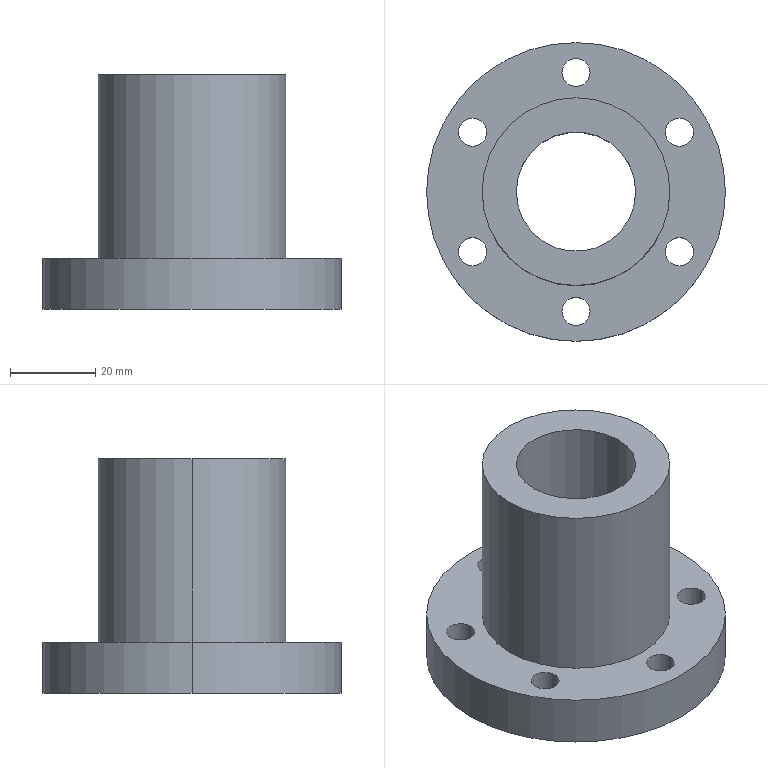Part | SolidWorks | features BaseBody 1 | 1 solid | 39 faces | box 70 x 70 x 55 mm | volume 72753 mm3 | cylinder 30 | plane 9 | commonest cylinder face diameters 6.6 x12 11 x12 28 x2 44 x2 70 x2
STEP:
#1=CARTESIAN_POINT('',(-24.249,19.5,6.8));
#2=VERTEX_POINT('',#1);
#3=CARTESIAN_POINT('',(-24.249,8.5,6.8));
#4=VERTEX_POINT('',#3);
#5=CARTESIAN_POINT('',(-24.249,14.,6.8));
#6=DIRECTION('',(0.,0.,1.));
#7=DIRECTION('',(0.,1.,0.));
#8=AXIS2_PLACEMENT_3D('',#5,#6,#7);
#9=CIRCLE('',#8,5.5);
#10=EDGE_CURVE('',#2,#4,#9,.T.);
#11=ORIENTED_EDGE('',*,*,#10,.T.);
#12=CARTESIAN_POINT('',(-24.249,8.5,0.));
#13=VERTEX_POINT('',#12);
#14=CARTESIAN_POINT('',(-24.249,8.5,6.8));
#15=DIRECTION('',(0.,0.,-1.));
#16=VECTOR('',#15,1000.);
#17=LINE('',#14,#16);
#18=EDGE_CURVE('',#4,#13,#17,.T.);
#19=ORIENTED_EDGE('',*,*,#18,.T.);
#20=CARTESIAN_POINT('',(-24.249,19.5,0.));
#21=VERTEX_POINT('',#20);
#22=CARTESIAN_POINT('',(-24.249,14.,0.));
#23=DIRECTION('',(0.,0.,-1.));
#24=DIRECTION('',(0.,1.,0.));
#25=AXIS2_PLACEMENT_3D('',#22,#23,#24);
#26=CIRCLE('',#25,5.5);
#27=EDGE_CURVE('',#13,#21,#26,.T.);
#28=ORIENTED_EDGE('',*,*,#27,.T.);
#29=CARTESIAN_POINT('',(-24.249,19.5,6.8));
#30=DIRECTION('',(0.,0.,-1.));
#31=VECTOR('',#30,1000.);
#32=LINE('',#29,#31);
#33=EDGE_CURVE('',#2,#21,#32,.T.);
#34=ORIENTED_EDGE('',*,*,#33,.F.);
#35=EDGE_LOOP('',(#11,#19,#28,#34));
#36=FACE_OUTER_BOUND('',#35,.T.);
#37=CARTESIAN_POINT('',(-24.249,14.,6.8));
#38=DIRECTION('',(0.,0.,-1.));
#39=DIRECTION('',(0.,1.,0.));
#40=AXIS2_PLACEMENT_3D('',#37,#38,#39);
#41=CYLINDRICAL_SURFACE('',#40,5.5);
#42=ADVANCED_FACE('',(#36),#41,.F.);
#43=CARTESIAN_POINT('',(-14.,0.,55.));
#44=VERTEX_POINT('',#43);
#45=CARTESIAN_POINT('',(14.,0.,55.));
#46=VERTEX_POINT('',#45);
#47=CARTESIAN_POINT('',(0.,0.,55.));
#48=DIRECTION('',(0.,0.,1.));
#49=DIRECTION('',(-1.,0.,0.));
#50=AXIS2_PLACEMENT_3D('',#47,#48,#49);
#51=CIRCLE('',#50,14.);
#52=EDGE_CURVE('',#44,#46,#51,.T.);
#53=ORIENTED_EDGE('',*,*,#52,.T.);
#54=CARTESIAN_POINT('',(14.,0.,0.));
#55=VERTEX_POINT('',#54);
#56=CARTESIAN_POINT('',(14.,0.,55.));
#57=DIRECTION('',(0.,0.,-1.));
#58=VECTOR('',#57,1000.);
#59=LINE('',#56,#58);
#60=EDGE_CURVE('',#46,#55,#59,.T.);
#61=ORIENTED_EDGE('',*,*,#60,.T.);
#62=CARTESIAN_POINT('',(-14.,0.,0.));
#63=VERTEX_POINT('',#62);
#64=CARTESIAN_POINT('',(0.,0.,0.));
#65=DIRECTION('',(0.,0.,-1.));
#66=DIRECTION('',(-1.,0.,0.));
#67=AXIS2_PLACEMENT_3D('',#64,#65,#66);
#68=CIRCLE('',#67,14.);
#69=EDGE_CURVE('',#55,#63,#68,.T.);
#70=ORIENTED_EDGE('',*,*,#69,.T.);
#71=CARTESIAN_POINT('',(-14.,0.,55.));
#72=DIRECTION('',(0.,0.,-1.));
#73=VECTOR('',#72,1000.);
#74=LINE('',#71,#73);
#75=EDGE_CURVE('',#44,#63,#74,.T.);
#76=ORIENTED_EDGE('',*,*,#75,.F.);
#77=EDGE_LOOP('',(#53,#61,#70,#76));
#78=FACE_OUTER_BOUND('',#77,.T.);
#79=CARTESIAN_POINT('',(0.,0.,55.));
#80=DIRECTION('',(0.,0.,-1.));
#81=DIRECTION('',(-1.,0.,0.));
#82=AXIS2_PLACEMENT_3D('',#79,#80,#81);
#83=CYLINDRICAL_SURFACE('',#82,14.);
#84=ADVANCED_FACE('',(#78),#83,.F.);
#85=CARTESIAN_POINT('',(0.,33.5,6.8));
#86=VERTEX_POINT('',#85);
#87=CARTESIAN_POINT('',(0.,22.5,6.8));
#88=VERTEX_POINT('',#87);
#89=CARTESIAN_POINT('',(0.,28.,6.8));
#90=DIRECTION('',(0.,0.,1.));
#91=DIRECTION('',(0.,1.,0.));
#92=AXIS2_PLACEMENT_3D('',#89,#90,#91);
#93=CIRCLE('',#92,5.5);
#94=EDGE_CURVE('',#86,#88,#93,.T.);
#95=ORIENTED_EDGE('',*,*,#94,.T.);
#96=CARTESIAN_POINT('',(0.,22.5,0.));
#97=VERTEX_POINT('',#96);
#98=CARTESIAN_POINT('',(0.,22.5,6.8));
#99=DIRECTION('',(0.,0.,-1.));
#100=VECTOR('',#99,1000.);
#101=LINE('',#98,#100);
#102=EDGE_CURVE('',#88,#97,#101,.T.);
#103=ORIENTED_EDGE('',*,*,#102,.T.);
#104=CARTESIAN_POINT('',(0.,33.5,0.));
#105=VERTEX_POINT('',#104);
#106=CARTESIAN_POINT('',(0.,28.,0.));
#107=DIRECTION('',(0.,0.,-1.));
#108=DIRECTION('',(0.,1.,0.));
#109=AXIS2_PLACEMENT_3D('',#106,#107,#108);
#110=CIRCLE('',#109,5.5);
#111=EDGE_CURVE('',#97,#105,#110,.T.);
#112=ORIENTED_EDGE('',*,*,#111,.T.);
#113=CARTESIAN_POINT('',(0.,33.5,6.8));
#114=DIRECTION('',(0.,0.,-1.));
#115=VECTOR('',#114,1000.);
#116=LINE('',#113,#115);
#117=EDGE_CURVE('',#86,#105,#116,.T.);
#118=ORIENTED_EDGE('',*,*,#117,.F.);
#119=EDGE_LOOP('',(#95,#103,#112,#118));
#120=FACE_OUTER_BOUND('',#119,.T.);
#121=CARTESIAN_POINT('',(0.,28.,6.8));
#122=DIRECTION('',(0.,0.,-1.));
#123=DIRECTION('',(0.,1.,0.));
#124=AXIS2_PLACEMENT_3D('',#121,#122,#123);
#125=CYLINDRICAL_SURFACE('',#124,5.5);
#126=ADVANCED_FACE('',(#120),#125,.F.);
#127=CARTESIAN_POINT('',(24.249,19.5,6.8));
#128=VERTEX_POINT('',#127);
#129=CARTESIAN_POINT('',(24.249,8.5,6.8));
#130=VERTEX_POINT('',#129);
#131=CARTESIAN_POINT('',(24.249,14.,6.8));
#132=DIRECTION('',(0.,0.,1.));
#133=DIRECTION('',(0.,1.,0.));
#134=AXIS2_PLACEMENT_3D('',#131,#132,#133);
#135=CIRCLE('',#134,5.5);
#136=EDGE_CURVE('',#128,#130,#135,.T.);
#137=ORIENTED_EDGE('',*,*,#136,.T.);
#138=CARTESIAN_POINT('',(24.249,8.5,0.));
#139=VERTEX_POINT('',#138);
#140=CARTESIAN_POINT('',(24.249,8.5,6.8));
#141=DIRECTION('',(0.,0.,-1.));
#142=VECTOR('',#141,1000.);
#143=LINE('',#140,#142);
#144=EDGE_CURVE('',#130,#139,#143,.T.);
#145=ORIENTED_EDGE('',*,*,#144,.T.);
#146=CARTESIAN_POINT('',(24.249,19.5,0.));
#147=VERTEX_POINT('',#146);
#148=CARTESIAN_POINT('',(24.249,14.,0.));
#149=DIRECTION('',(0.,0.,-1.));
#150=DIRECTION('',(0.,1.,0.));
#151=AXIS2_PLACEMENT_3D('',#148,#149,#150);
#152=CIRCLE('',#151,5.5);
#153=EDGE_CURVE('',#139,#147,#152,.T.);
#154=ORIENTED_EDGE('',*,*,#153,.T.);
#155=CARTESIAN_POINT('',(24.249,19.5,6.8));
#156=DIRECTION('',(0.,0.,-1.));
#157=VECTOR('',#156,1000.);
#158=LINE('',#155,#157);
#159=EDGE_CURVE('',#128,#147,#158,.T.);
#160=ORIENTED_EDGE('',*,*,#159,.F.);
#161=EDGE_LOOP('',(#137,#145,#154,#160));
#162=FACE_OUTER_BOUND('',#161,.T.);
#163=CARTESIAN_POINT('',(24.249,14.,6.8));
#164=DIRECTION('',(0.,0.,-1.));
#165=DIRECTION('',(0.,1.,0.));
#166=AXIS2_PLACEMENT_3D('',#163,#164,#165);
#167=CYLINDRICAL_SURFACE('',#166,5.5);
#168=ADVANCED_FACE('',(#162),#167,.F.);
#169=CARTESIAN_POINT('',(24.249,-8.5,6.8));
#170=VERTEX_POINT('',#169);
#171=CARTESIAN_POINT('',(24.249,-19.5,6.8));
#172=VERTEX_POINT('',#171);
#173=CARTESIAN_POINT('',(24.249,-14.,6.8));
#174=DIRECTION('',(0.,0.,1.));
#175=DIRECTION('',(0.,1.,0.));
#176=AXIS2_PLACEMENT_3D('',#173,#174,#175);
#177=CIRCLE('',#176,5.5);
#178=EDGE_CURVE('',#170,#172,#177,.T.);
#179=ORIENTED_EDGE('',*,*,#178,.T.);
#180=CARTESIAN_POINT('',(24.249,-19.5,0.));
#181=VERTEX_POINT('',#180);
#182=CARTESIAN_POINT('',(24.249,-19.5,6.8));
#183=DIRECTION('',(0.,0.,-1.));
#184=VECTOR('',#183,1000.);
#185=LINE('',#182,#184);
#186=EDGE_CURVE('',#172,#181,#185,.T.);
#187=ORIENTED_EDGE('',*,*,#186,.T.);
#188=CARTESIAN_POINT('',(24.249,-8.5,0.));
#189=VERTEX_POINT('',#188);
#190=CARTESIAN_POINT('',(24.249,-14.,0.));
#191=DIRECTION('',(0.,0.,-1.));
#192=DIRECTION('',(0.,1.,0.));
#193=AXIS2_PLACEMENT_3D('',#190,#191,#192);
#194=CIRCLE('',#193,5.5);
#195=EDGE_CURVE('',#181,#189,#194,.T.);
#196=ORIENTED_EDGE('',*,*,#195,.T.);
#197=CARTESIAN_POINT('',(24.249,-8.5,6.8));
#198=DIRECTION('',(0.,0.,-1.));
#199=VECTOR('',#198,1000.);
#200=LINE('',#197,#199);
#201=EDGE_CURVE('',#170,#189,#200,.T.);
#202=ORIENTED_EDGE('',*,*,#201,.F.);
#203=EDGE_LOOP('',(#179,#187,#196,#202));
#204=FACE_OUTER_BOUND('',#203,.T.);
#205=CARTESIAN_POINT('',(24.249,-14.,6.8));
#206=DIRECTION('',(0.,0.,-1.));
#207=DIRECTION('',(0.,1.,0.));
#208=AXIS2_PLACEMENT_3D('',#205,#206,#207);
#209=CYLINDRICAL_SURFACE('',#208,5.5);
#210=ADVANCED_FACE('',(#204),#209,.F.);
#211=CARTESIAN_POINT('',(0.,-22.5,6.8));
#212=VERTEX_POINT('',#211);
#213=CARTESIAN_POINT('',(0.,-33.5,6.8));
#214=VERTEX_POINT('',#213);
#215=CARTESIAN_POINT('',(0.,-28.,6.8));
#216=DIRECTION('',(0.,0.,1.));
#217=DIRECTION('',(0.,1.,0.));
#218=AXIS2_PLACEMENT_3D('',#215,#216,#217);
#219=CIRCLE('',#218,5.5);
#220=EDGE_CURVE('',#212,#214,#219,.T.);
#221=ORIENTED_EDGE('',*,*,#220,.T.);
#222=CARTESIAN_POINT('',(0.,-33.5,0.));
#223=VERTEX_POINT('',#222);
#224=CARTESIAN_POINT('',(0.,-33.5,6.8));
#225=DIRECTION('',(0.,0.,-1.));
#226=VECTOR('',#225,1000.);
#227=LINE('',#224,#226);
#228=EDGE_CURVE('',#214,#223,#227,.T.);
#229=ORIENTED_EDGE('',*,*,#228,.T.);
#230=CARTESIAN_POINT('',(0.,-22.5,0.));
#231=VERTEX_POINT('',#230);
#232=CARTESIAN_POINT('',(0.,-28.,0.));
#233=DIRECTION('',(0.,0.,-1.));
#234=DIRECTION('',(0.,1.,0.));
#235=AXIS2_PLACEMENT_3D('',#232,#233,#234);
#236=CIRCLE('',#235,5.5);
#237=EDGE_CURVE('',#223,#231,#236,.T.);
#238=ORIENTED_EDGE('',*,*,#237,.T.);
#239=CARTESIAN_POINT('',(0.,-22.5,6.8));
#240=DIRECTION('',(0.,0.,-1.));
#241=VECTOR('',#240,1000.);
#242=LINE('',#239,#241);
#243=EDGE_CURVE('',#212,#231,#242,.T.);
#244=ORIENTED_EDGE('',*,*,#243,.F.);
#245=EDGE_LOOP('',(#221,#229,#238,#244));
#246=FACE_OUTER_BOUND('',#245,.T.);
#247=CARTESIAN_POINT('',(0.,-28.,6.8));
#248=DIRECTION('',(0.,0.,-1.));
#249=DIRECTION('',(0.,1.,0.));
#250=AXIS2_PLACEMENT_3D('',#247,#248,#249);
#251=CYLINDRICAL_SURFACE('',#250,5.5);
#252=ADVANCED_FACE('',(#246),#251,.F.);
#253=CARTESIAN_POINT('',(-24.249,-8.5,6.8));
#254=VERTEX_POINT('',#253);
#255=CARTESIAN_POINT('',(-24.249,-19.5,6.8));
#256=VERTEX_POINT('',#255);
#257=CARTESIAN_POINT('',(-24.249,-14.,6.8));
#258=DIRECTION('',(0.,0.,1.));
#259=DIRECTION('',(0.,1.,0.));
#260=AXIS2_PLACEMENT_3D('',#257,#258,#259);
#261=CIRCLE('',#260,5.5);
#262=EDGE_CURVE('',#254,#256,#261,.T.);
#263=ORIENTED_EDGE('',*,*,#262,.T.);
#264=CARTESIAN_POINT('',(-24.249,-19.5,0.));
#265=VERTEX_POINT('',#264);
#266=CARTESIAN_POINT('',(-24.249,-19.5,6.8));
#267=DIRECTION('',(0.,0.,-1.));
#268=VECTOR('',#267,1000.);
#269=LINE('',#266,#268);
#270=EDGE_CURVE('',#256,#265,#269,.T.);
#271=ORIENTED_EDGE('',*,*,#270,.T.);
#272=CARTESIAN_POINT('',(-24.249,-8.5,0.));
#273=VERTEX_POINT('',#272);
#274=CARTESIAN_POINT('',(-24.249,-14.,0.));
#275=DIRECTION('',(0.,0.,-1.));
#276=DIRECTION('',(0.,1.,0.));
#277=AXIS2_PLACEMENT_3D('',#274,#275,#276);
#278=CIRCLE('',#277,5.5);
#279=EDGE_CURVE('',#265,#273,#278,.T.);
#280=ORIENTED_EDGE('',*,*,#279,.T.);
#281=CARTESIAN_POINT('',(-24.249,-8.5,6.8));
#282=DIRECTION('',(0.,0.,-1.));
#283=VECTOR('',#282,1000.);
#284=LINE('',#281,#283);
#285=EDGE_CURVE('',#254,#273,#284,.T.);
#286=ORIENTED_EDGE('',*,*,#285,.F.);
#287=EDGE_LOOP('',(#263,#271,#280,#286));
#288=FACE_OUTER_BOUND('',#287,.T.);
#289=CARTESIAN_POINT('',(-24.249,-14.,6.8));
#290=DIRECTION('',(0.,0.,-1.));
#291=DIRECTION('',(0.,1.,0.));
#292=AXIS2_PLACEMENT_3D('',#289,#290,#291);
#293=CYLINDRICAL_SURFACE('',#292,5.5);
#294=ADVANCED_FACE('',(#288),#293,.F.);
#295=CARTESIAN_POINT('',(35.,0.,12.));
#296=VERTEX_POINT('',#295);
#297=CARTESIAN_POINT('',(-35.,0.,12.));
#298=VERTEX_POINT('',#297);
#299=CARTESIAN_POINT('',(0.,0.,12.));
#300=DIRECTION('',(0.,0.,1.));
#301=DIRECTION('',(-1.,0.,0.));
#302=AXIS2_PLACEMENT_3D('',#299,#300,#301);
#303=CIRCLE('',#302,35.);
#304=EDGE_CURVE('',#296,#298,#303,.T.);
#305=ORIENTED_EDGE('',*,*,#304,.F.);
#306=CARTESIAN_POINT('',(35.,0.,0.));
#307=VERTEX_POINT('',#306);
#308=CARTESIAN_POINT('',(35.,0.,12.));
#309=DIRECTION('',(0.,0.,-1.));
#310=VECTOR('',#309,1000.);
#311=LINE('',#308,#310);
#312=EDGE_CURVE('',#296,#307,#311,.T.);
#313=ORIENTED_EDGE('',*,*,#312,.T.);
#314=CARTESIAN_POINT('',(-35.,0.,0.));
#315=VERTEX_POINT('',#314);
#316=CARTESIAN_POINT('',(0.,0.,0.));
#317=DIRECTION('',(0.,0.,1.));
#318=DIRECTION('',(-1.,0.,0.));
#319=AXIS2_PLACEMENT_3D('',#316,#317,#318);
#320=CIRCLE('',#319,35.);
#321=EDGE_CURVE('',#307,#315,#320,.T.);
#322=ORIENTED_EDGE('',*,*,#321,.T.);
#323=CARTESIAN_POINT('',(-35.,0.,12.));
#324=DIRECTION('',(0.,0.,-1.));
#325=VECTOR('',#324,1000.);
#326=LINE('',#323,#325);
#327=EDGE_CURVE('',#298,#315,#326,.T.);
#328=ORIENTED_EDGE('',*,*,#327,.F.);
#329=EDGE_LOOP('',(#305,#313,#322,#328));
#330=FACE_OUTER_BOUND('',#329,.T.);
#331=CARTESIAN_POINT('',(0.,0.,12.));
#332=DIRECTION('',(0.,0.,-1.));
#333=DIRECTION('',(-1.,0.,0.));
#334=AXIS2_PLACEMENT_3D('',#331,#332,#333);
#335=CYLINDRICAL_SURFACE('',#334,35.);
#336=ADVANCED_FACE('',(#330),#335,.T.);
#337=CARTESIAN_POINT('',(-27.549,14.,12.));
#338=VERTEX_POINT('',#337);
#339=CARTESIAN_POINT('',(-20.949,14.,12.));
#340=VERTEX_POINT('',#339);
#341=CARTESIAN_POINT('',(-24.249,14.,12.));
#342=DIRECTION('',(0.,0.,1.));
#343=DIRECTION('',(-1.,0.,0.));
#344=AXIS2_PLACEMENT_3D('',#341,#342,#343);
#345=CIRCLE('',#344,3.3);
#346=EDGE_CURVE('',#338,#340,#345,.T.);
#347=ORIENTED_EDGE('',*,*,#346,.T.);
#348=CARTESIAN_POINT('',(-20.949,14.,6.8));
#349=VERTEX_POINT('',#348);
#350=CARTESIAN_POINT('',(-20.949,14.,12.));
#351=DIRECTION('',(0.,0.,-1.));
#352=VECTOR('',#351,1000.);
#353=LINE('',#350,#352);
#354=EDGE_CURVE('',#340,#349,#353,.T.);
#355=ORIENTED_EDGE('',*,*,#354,.T.);
#356=CARTESIAN_POINT('',(-27.549,14.,6.8));
#357=VERTEX_POINT('',#356);
#358=CARTESIAN_POINT('',(-24.249,14.,6.8));
#359=DIRECTION('',(0.,0.,-1.));
#360=DIRECTION('',(-1.,0.,0.));
#361=AXIS2_PLACEMENT_3D('',#358,#359,#360);
#362=CIRCLE('',#361,3.3);
#363=EDGE_CURVE('',#349,#357,#362,.T.);
#364=ORIENTED_EDGE('',*,*,#363,.T.);
#365=CARTESIAN_POINT('',(-27.549,14.,12.));
#366=DIRECTION('',(0.,0.,-1.));
#367=VECTOR('',#366,1000.);
#368=LINE('',#365,#367);
#369=EDGE_CURVE('',#338,#357,#368,.T.);
#370=ORIENTED_EDGE('',*,*,#369,.F.);
#371=EDGE_LOOP('',(#347,#355,#364,#370));
#372=FACE_OUTER_BOUND('',#371,.T.);
#373=CARTESIAN_POINT('',(-24.249,14.,12.));
#374=DIRECTION('',(0.,0.,-1.));
#375=DIRECTION('',(-1.,0.,0.));
#376=AXIS2_PLACEMENT_3D('',#373,#374,#375);
#377=CYLINDRICAL_SURFACE('',#376,3.3);
#378=ADVANCED_FACE('',(#372),#377,.F.);
#379=CARTESIAN_POINT('',(22.,0.,55.));
#380=VERTEX_POINT('',#379);
#381=CARTESIAN_POINT('',(-22.,0.,55.));
#382=VERTEX_POINT('',#381);
#383=CARTESIAN_POINT('',(0.,0.,55.));
#384=DIRECTION('',(0.,0.,1.));
#385=DIRECTION('',(-1.,0.,0.));
#386=AXIS2_PLACEMENT_3D('',#383,#384,#385);
#387=CIRCLE('',#386,22.);
#388=EDGE_CURVE('',#380,#382,#387,.T.);
#389=ORIENTED_EDGE('',*,*,#388,.F.);
#390=CARTESIAN_POINT('',(22.,0.,12.));
#391=VERTEX_POINT('',#390);
#392=CARTESIAN_POINT('',(22.,0.,55.));
#393=DIRECTION('',(0.,0.,-1.));
#394=VECTOR('',#393,1000.);
#395=LINE('',#392,#394);
#396=EDGE_CURVE('',#380,#391,#395,.T.);
#397=ORIENTED_EDGE('',*,*,#396,.T.);
#398=CARTESIAN_POINT('',(-22.,0.,12.));
#399=VERTEX_POINT('',#398);
#400=CARTESIAN_POINT('',(0.,0.,12.));
#401=DIRECTION('',(0.,0.,-1.));
#402=DIRECTION('',(-1.,0.,0.));
#403=AXIS2_PLACEMENT_3D('',#400,#401,#402);
#404=CIRCLE('',#403,22.);
#405=EDGE_CURVE('',#399,#391,#404,.T.);
#406=ORIENTED_EDGE('',*,*,#405,.F.);
#407=CARTESIAN_POINT('',(-22.,0.,55.));
#408=DIRECTION('',(0.,0.,-1.));
#409=VECTOR('',#408,1000.);
#410=LINE('',#407,#409);
#411=EDGE_CURVE('',#382,#399,#410,.T.);
#412=ORIENTED_EDGE('',*,*,#411,.F.);
#413=EDGE_LOOP('',(#389,#397,#406,#412));
#414=FACE_OUTER_BOUND('',#413,.T.);
#415=CARTESIAN_POINT('',(0.,0.,55.));
#416=DIRECTION('',(0.,0.,-1.));
#417=DIRECTION('',(-1.,0.,0.));
#418=AXIS2_PLACEMENT_3D('',#415,#416,#417);
#419=CYLINDRICAL_SURFACE('',#418,22.);
#420=ADVANCED_FACE('',(#414),#419,.T.);
#421=CARTESIAN_POINT('',(3.3,28.,12.));
#422=VERTEX_POINT('',#421);
#423=CARTESIAN_POINT('',(-3.3,28.,12.));
#424=VERTEX_POINT('',#423);
#425=CARTESIAN_POINT('',(0.,28.,12.));
#426=DIRECTION('',(0.,0.,-1.));
#427=DIRECTION('',(-1.,0.,0.));
#428=AXIS2_PLACEMENT_3D('',#425,#426,#427);
#429=CIRCLE('',#428,3.3);
#430=EDGE_CURVE('',#422,#424,#429,.T.);
#431=ORIENTED_EDGE('',*,*,#430,.F.);
#432=CARTESIAN_POINT('',(3.3,28.,6.8));
#433=VERTEX_POINT('',#432);
#434=CARTESIAN_POINT('',(3.3,28.,12.));
#435=DIRECTION('',(0.,0.,-1.));
#436=VECTOR('',#435,1000.);
#437=LINE('',#434,#436);
#438=EDGE_CURVE('',#422,#433,#437,.T.);
#439=ORIENTED_EDGE('',*,*,#438,.T.);
#440=CARTESIAN_POINT('',(-3.3,28.,6.8));
#441=VERTEX_POINT('',#440);
#442=CARTESIAN_POINT('',(0.,28.,6.8));
#443=DIRECTION('',(0.,0.,-1.));
#444=DIRECTION('',(-1.,0.,0.));
#445=AXIS2_PLACEMENT_3D('',#442,#443,#444);
#446=CIRCLE('',#445,3.3);
#447=EDGE_CURVE('',#433,#441,#446,.T.);
#448=ORIENTED_EDGE('',*,*,#447,.T.);
#449=CARTESIAN_POINT('',(-3.3,28.,12.));
#450=DIRECTION('',(0.,0.,-1.));
#451=VECTOR('',#450,1000.);
#452=LINE('',#449,#451);
#453=EDGE_CURVE('',#424,#441,#452,.T.);
#454=ORIENTED_EDGE('',*,*,#453,.F.);
#455=EDGE_LOOP('',(#431,#439,#448,#454));
#456=FACE_OUTER_BOUND('',#455,.T.);
#457=CARTESIAN_POINT('',(0.,28.,12.));
#458=DIRECTION('',(0.,0.,-1.));
#459=DIRECTION('',(-1.,0.,0.));
#460=AXIS2_PLACEMENT_3D('',#457,#458,#459);
#461=CYLINDRICAL_SURFACE('',#460,3.3);
#462=ADVANCED_FACE('',(#456),#461,.F.);
#463=CARTESIAN_POINT('',(27.549,14.,12.));
#464=VERTEX_POINT('',#463);
#465=CARTESIAN_POINT('',(20.949,14.,12.));
#466=VERTEX_POINT('',#465);
#467=CARTESIAN_POINT('',(24.249,14.,12.));
#468=DIRECTION('',(0.,0.,-1.));
#469=DIRECTION('',(-1.,0.,0.));
#470=AXIS2_PLACEMENT_3D('',#467,#468,#469);
#471=CIRCLE('',#470,3.3);
#472=EDGE_CURVE('',#464,#466,#471,.T.);
#473=ORIENTED_EDGE('',*,*,#472,.F.);
#474=CARTESIAN_POINT('',(27.549,14.,6.8));
#475=VERTEX_POINT('',#474);
#476=CARTESIAN_POINT('',(27.549,14.,12.));
#477=DIRECTION('',(0.,0.,-1.));
#478=VECTOR('',#477,1000.);
#479=LINE('',#476,#478);
#480=EDGE_CURVE('',#464,#475,#479,.T.);
#481=ORIENTED_EDGE('',*,*,#480,.T.);
#482=CARTESIAN_POINT('',(20.949,14.,6.8));
#483=VERTEX_POINT('',#482);
#484=CARTESIAN_POINT('',(24.249,14.,6.8));
#485=DIRECTION('',(0.,0.,-1.));
#486=DIRECTION('',(-1.,0.,0.));
#487=AXIS2_PLACEMENT_3D('',#484,#485,#486);
#488=CIRCLE('',#487,3.3);
#489=EDGE_CURVE('',#475,#483,#488,.T.);
#490=ORIENTED_EDGE('',*,*,#489,.T.);
#491=CARTESIAN_POINT('',(20.949,14.,12.));
#492=DIRECTION('',(0.,0.,-1.));
#493=VECTOR('',#492,1000.);
#494=LINE('',#491,#493);
#495=EDGE_CURVE('',#466,#483,#494,.T.);
#496=ORIENTED_EDGE('',*,*,#495,.F.);
#497=EDGE_LOOP('',(#473,#481,#490,#496));
#498=FACE_OUTER_BOUND('',#497,.T.);
#499=CARTESIAN_POINT('',(24.249,14.,12.));
#500=DIRECTION('',(0.,0.,-1.));
#501=DIRECTION('',(-1.,0.,0.));
#502=AXIS2_PLACEMENT_3D('',#499,#500,#501);
#503=CYLINDRICAL_SURFACE('',#502,3.3);
#504=ADVANCED_FACE('',(#498),#503,.F.);
#505=CARTESIAN_POINT('',(27.549,-14.,12.));
#506=VERTEX_POINT('',#505);
#507=CARTESIAN_POINT('',(20.949,-14.,12.));
#508=VERTEX_POINT('',#507);
#509=CARTESIAN_POINT('',(24.249,-14.,12.));
#510=DIRECTION('',(0.,0.,-1.));
#511=DIRECTION('',(-1.,0.,0.));
#512=AXIS2_PLACEMENT_3D('',#509,#510,#511);
#513=CIRCLE('',#512,3.3);
#514=EDGE_CURVE('',#506,#508,#513,.T.);
#515=ORIENTED_EDGE('',*,*,#514,.F.);
#516=CARTESIAN_POINT('',(27.549,-14.,6.8));
#517=VERTEX_POINT('',#516);
#518=CARTESIAN_POINT('',(27.549,-14.,12.));
#519=DIRECTION('',(0.,0.,-1.));
#520=VECTOR('',#519,1000.);
#521=LINE('',#518,#520);
#522=EDGE_CURVE('',#506,#517,#521,.T.);
#523=ORIENTED_EDGE('',*,*,#522,.T.);
#524=CARTESIAN_POINT('',(20.949,-14.,6.8));
#525=VERTEX_POINT('',#524);
#526=CARTESIAN_POINT('',(24.249,-14.,6.8));
#527=DIRECTION('',(0.,0.,-1.));
#528=DIRECTION('',(-1.,0.,0.));
#529=AXIS2_PLACEMENT_3D('',#526,#527,#528);
#530=CIRCLE('',#529,3.3);
#531=EDGE_CURVE('',#517,#525,#530,.T.);
#532=ORIENTED_EDGE('',*,*,#531,.T.);
#533=CARTESIAN_POINT('',(20.949,-14.,12.));
#534=DIRECTION('',(0.,0.,-1.));
#535=VECTOR('',#534,1000.);
#536=LINE('',#533,#535);
#537=EDGE_CURVE('',#508,#525,#536,.T.);
#538=ORIENTED_EDGE('',*,*,#537,.F.);
#539=EDGE_LOOP('',(#515,#523,#532,#538));
#540=FACE_OUTER_BOUND('',#539,.T.);
#541=CARTESIAN_POINT('',(24.249,-14.,12.));
#542=DIRECTION('',(0.,0.,-1.));
#543=DIRECTION('',(-1.,0.,0.));
#544=AXIS2_PLACEMENT_3D('',#541,#542,#543);
#545=CYLINDRICAL_SURFACE('',#544,3.3);
#546=ADVANCED_FACE('',(#540),#545,.F.);
#547=CARTESIAN_POINT('',(3.3,-28.,12.));
#548=VERTEX_POINT('',#547);
#549=CARTESIAN_POINT('',(-3.3,-28.,12.));
#550=VERTEX_POINT('',#549);
#551=CARTESIAN_POINT('',(0.,-28.,12.));
#552=DIRECTION('',(0.,0.,-1.));
#553=DIRECTION('',(-1.,0.,0.));
#554=AXIS2_PLACEMENT_3D('',#551,#552,#553);
#555=CIRCLE('',#554,3.3);
#556=EDGE_CURVE('',#548,#550,#555,.T.);
#557=ORIENTED_EDGE('',*,*,#556,.F.);
#558=CARTESIAN_POINT('',(3.3,-28.,6.8));
#559=VERTEX_POINT('',#558);
#560=CARTESIAN_POINT('',(3.3,-28.,12.));
#561=DIRECTION('',(0.,0.,-1.));
#562=VECTOR('',#561,1000.);
#563=LINE('',#560,#562);
#564=EDGE_CURVE('',#548,#559,#563,.T.);
#565=ORIENTED_EDGE('',*,*,#564,.T.);
#566=CARTESIAN_POINT('',(-3.3,-28.,6.8));
#567=VERTEX_POINT('',#566);
#568=CARTESIAN_POINT('',(0.,-28.,6.8));
#569=DIRECTION('',(0.,0.,-1.));
#570=DIRECTION('',(-1.,0.,0.));
#571=AXIS2_PLACEMENT_3D('',#568,#569,#570);
#572=CIRCLE('',#571,3.3);
#573=EDGE_CURVE('',#559,#567,#572,.T.);
#574=ORIENTED_EDGE('',*,*,#573,.T.);
#575=CARTESIAN_POINT('',(-3.3,-28.,12.));
#576=DIRECTION('',(0.,0.,-1.));
#577=VECTOR('',#576,1000.);
#578=LINE('',#575,#577);
#579=EDGE_CURVE('',#550,#567,#578,.T.);
#580=ORIENTED_EDGE('',*,*,#579,.F.);
#581=EDGE_LOOP('',(#557,#565,#574,#580));
#582=FACE_OUTER_BOUND('',#581,.T.);
#583=CARTESIAN_POINT('',(0.,-28.,12.));
#584=DIRECTION('',(0.,0.,-1.));
#585=DIRECTION('',(-1.,0.,0.));
#586=AXIS2_PLACEMENT_3D('',#583,#584,#585);
#587=CYLINDRICAL_SURFACE('',#586,3.3);
#588=ADVANCED_FACE('',(#582),#587,.F.);
#589=CARTESIAN_POINT('',(-20.949,-14.,12.));
#590=VERTEX_POINT('',#589);
#591=CARTESIAN_POINT('',(-27.549,-14.,12.));
#592=VERTEX_POINT('',#591);
#593=CARTESIAN_POINT('',(-24.249,-14.,12.));
#594=DIRECTION('',(0.,0.,-1.));
#595=DIRECTION('',(-1.,0.,0.));
#596=AXIS2_PLACEMENT_3D('',#593,#594,#595);
#597=CIRCLE('',#596,3.3);
#598=EDGE_CURVE('',#590,#592,#597,.T.);
#599=ORIENTED_EDGE('',*,*,#598,.F.);
#600=CARTESIAN_POINT('',(-20.949,-14.,6.8));
#601=VERTEX_POINT('',#600);
#602=CARTESIAN_POINT('',(-20.949,-14.,12.));
#603=DIRECTION('',(0.,0.,-1.));
#604=VECTOR('',#603,1000.);
#605=LINE('',#602,#604);
#606=EDGE_CURVE('',#590,#601,#605,.T.);
#607=ORIENTED_EDGE('',*,*,#606,.T.);
#608=CARTESIAN_POINT('',(-27.549,-14.,6.8));
#609=VERTEX_POINT('',#608);
#610=CARTESIAN_POINT('',(-24.249,-14.,6.8));
#611=DIRECTION('',(0.,0.,-1.));
#612=DIRECTION('',(-1.,0.,0.));
#613=AXIS2_PLACEMENT_3D('',#610,#611,#612);
#614=CIRCLE('',#613,3.3);
#615=EDGE_CURVE('',#601,#609,#614,.T.);
#616=ORIENTED_EDGE('',*,*,#615,.T.);
#617=CARTESIAN_POINT('',(-27.549,-14.,12.));
#618=DIRECTION('',(0.,0.,-1.));
#619=VECTOR('',#618,1000.);
#620=LINE('',#617,#619);
#621=EDGE_CURVE('',#592,#609,#620,.T.);
#622=ORIENTED_EDGE('',*,*,#621,.F.);
#623=EDGE_LOOP('',(#599,#607,#616,#622));
#624=FACE_OUTER_BOUND('',#623,.T.);
#625=CARTESIAN_POINT('',(-24.249,-14.,12.));
#626=DIRECTION('',(0.,0.,-1.));
#627=DIRECTION('',(-1.,0.,0.));
#628=AXIS2_PLACEMENT_3D('',#625,#626,#627);
#629=CYLINDRICAL_SURFACE('',#628,3.3);
#630=ADVANCED_FACE('',(#624),#629,.F.);
#631=ORIENTED_EDGE('',*,*,#18,.F.);
#632=CARTESIAN_POINT('',(-24.249,14.,6.8));
#633=DIRECTION('',(0.,0.,1.));
#634=DIRECTION('',(0.,1.,0.));
#635=AXIS2_PLACEMENT_3D('',#632,#633,#634);
#636=CIRCLE('',#635,5.5);
#637=EDGE_CURVE('',#4,#2,#636,.T.);
#638=ORIENTED_EDGE('',*,*,#637,.T.);
#639=ORIENTED_EDGE('',*,*,#33,.T.);
#640=CARTESIAN_POINT('',(-24.249,14.,0.));
#641=DIRECTION('',(0.,0.,-1.));
#642=DIRECTION('',(0.,1.,0.));
#643=AXIS2_PLACEMENT_3D('',#640,#641,#642);
#644=CIRCLE('',#643,5.5);
#645=EDGE_CURVE('',#21,#13,#644,.T.);
#646=ORIENTED_EDGE('',*,*,#645,.T.);
#647=EDGE_LOOP('',(#631,#638,#639,#646));
#648=FACE_OUTER_BOUND('',#647,.T.);
#649=CARTESIAN_POINT('',(-24.249,14.,6.8));
#650=DIRECTION('',(0.,0.,-1.));
#651=DIRECTION('',(0.,1.,0.));
#652=AXIS2_PLACEMENT_3D('',#649,#650,#651);
#653=CYLINDRICAL_SURFACE('',#652,5.5);
#654=ADVANCED_FACE('',(#648),#653,.F.);
#655=CARTESIAN_POINT('',(0.,0.,0.));
#656=DIRECTION('',(0.,0.,-1.));
#657=DIRECTION('',(-1.,0.,0.));
#658=AXIS2_PLACEMENT_3D('',#655,#656,#657);
#659=CIRCLE('',#658,14.);
#660=EDGE_CURVE('',#63,#55,#659,.T.);
#661=ORIENTED_EDGE('',*,*,#660,.F.);
#662=ORIENTED_EDGE('',*,*,#69,.F.);
#663=EDGE_LOOP('',(#661,#662));
#664=FACE_BOUND('',#663,.T.);
#665=CARTESIAN_POINT('',(0.,28.,0.));
#666=DIRECTION('',(0.,0.,-1.));
#667=DIRECTION('',(0.,1.,0.));
#668=AXIS2_PLACEMENT_3D('',#665,#666,#667);
#669=CIRCLE('',#668,5.5);
#670=EDGE_CURVE('',#105,#97,#669,.T.);
#671=ORIENTED_EDGE('',*,*,#670,.F.);
#672=ORIENTED_EDGE('',*,*,#111,.F.);
#673=EDGE_LOOP('',(#671,#672));
#674=FACE_BOUND('',#673,.T.);
#675=CARTESIAN_POINT('',(24.249,14.,0.));
#676=DIRECTION('',(0.,0.,-1.));
#677=DIRECTION('',(0.,1.,0.));
#678=AXIS2_PLACEMENT_3D('',#675,#676,#677);
#679=CIRCLE('',#678,5.5);
#680=EDGE_CURVE('',#147,#139,#679,.T.);
#681=ORIENTED_EDGE('',*,*,#680,.F.);
#682=ORIENTED_EDGE('',*,*,#153,.F.);
#683=EDGE_LOOP('',(#681,#682));
#684=FACE_BOUND('',#683,.T.);
#685=CARTESIAN_POINT('',(24.249,-14.,0.));
#686=DIRECTION('',(0.,0.,-1.));
#687=DIRECTION('',(0.,1.,0.));
#688=AXIS2_PLACEMENT_3D('',#685,#686,#687);
#689=CIRCLE('',#688,5.5);
#690=EDGE_CURVE('',#189,#181,#689,.T.);
#691=ORIENTED_EDGE('',*,*,#690,.F.);
#692=ORIENTED_EDGE('',*,*,#195,.F.);
#693=EDGE_LOOP('',(#691,#692));
#694=FACE_BOUND('',#693,.T.);
#695=CARTESIAN_POINT('',(0.,-28.,0.));
#696=DIRECTION('',(0.,0.,-1.));
#697=DIRECTION('',(0.,1.,0.));
#698=AXIS2_PLACEMENT_3D('',#695,#696,#697);
#699=CIRCLE('',#698,5.5);
#700=EDGE_CURVE('',#231,#223,#699,.T.);
#701=ORIENTED_EDGE('',*,*,#700,.F.);
#702=ORIENTED_EDGE('',*,*,#237,.F.);
#703=EDGE_LOOP('',(#701,#702));
#704=FACE_BOUND('',#703,.T.);
#705=CARTESIAN_POINT('',(-24.249,-14.,0.));
#706=DIRECTION('',(0.,0.,-1.));
#707=DIRECTION('',(0.,1.,0.));
#708=AXIS2_PLACEMENT_3D('',#705,#706,#707);
#709=CIRCLE('',#708,5.5);
#710=EDGE_CURVE('',#273,#265,#709,.T.);
#711=ORIENTED_EDGE('',*,*,#710,.F.);
#712=ORIENTED_EDGE('',*,*,#279,.F.);
#713=EDGE_LOOP('',(#711,#712));
#714=FACE_BOUND('',#713,.T.);
#715=ORIENTED_EDGE('',*,*,#645,.F.);
#716=ORIENTED_EDGE('',*,*,#27,.F.);
#717=EDGE_LOOP('',(#715,#716));
#718=FACE_BOUND('',#717,.T.);
#719=CARTESIAN_POINT('',(0.,0.,0.));
#720=DIRECTION('',(0.,0.,1.));
#721=DIRECTION('',(-1.,0.,0.));
#722=AXIS2_PLACEMENT_3D('',#719,#720,#721);
#723=CIRCLE('',#722,35.);
#724=EDGE_CURVE('',#315,#307,#723,.T.);
#725=ORIENTED_EDGE('',*,*,#724,.F.);
#726=ORIENTED_EDGE('',*,*,#321,.F.);
#727=EDGE_LOOP('',(#725,#726));
#728=FACE_OUTER_BOUND('',#727,.T.);
#729=CARTESIAN_POINT('',(-35.42,-35.42,0.));
#730=DIRECTION('',(0.,0.,1.));
#731=DIRECTION('',(1.,0.,0.));
#732=AXIS2_PLACEMENT_3D('',#729,#730,#731);
#733=PLANE('',#732);
#734=ADVANCED_FACE('',(#664,#674,#684,#694,#704,#714,#718,#728),#733,.F.);
#735=CARTESIAN_POINT('',(-24.249,14.,6.8));
#736=DIRECTION('',(0.,0.,-1.));
#737=DIRECTION('',(-1.,0.,0.));
#738=AXIS2_PLACEMENT_3D('',#735,#736,#737);
#739=CIRCLE('',#738,3.3);
#740=EDGE_CURVE('',#357,#349,#739,.T.);
#741=ORIENTED_EDGE('',*,*,#740,.F.);
#742=ORIENTED_EDGE('',*,*,#363,.F.);
#743=EDGE_LOOP('',(#741,#742));
#744=FACE_BOUND('',#743,.T.);
#745=ORIENTED_EDGE('',*,*,#10,.F.);
#746=ORIENTED_EDGE('',*,*,#637,.F.);
#747=EDGE_LOOP('',(#745,#746));
#748=FACE_OUTER_BOUND('',#747,.T.);
#749=CARTESIAN_POINT('',(-29.815,8.434,6.8));
#750=DIRECTION('',(0.,0.,1.));
#751=DIRECTION('',(1.,0.,0.));
#752=AXIS2_PLACEMENT_3D('',#749,#750,#751);
#753=PLANE('',#752);
#754=ADVANCED_FACE('',(#744,#748),#753,.F.);
#755=ORIENTED_EDGE('',*,*,#60,.F.);
#756=CARTESIAN_POINT('',(0.,0.,55.));
#757=DIRECTION('',(0.,0.,1.));
#758=DIRECTION('',(-1.,0.,0.));
#759=AXIS2_PLACEMENT_3D('',#756,#757,#758);
#760=CIRCLE('',#759,14.);
#761=EDGE_CURVE('',#46,#44,#760,.T.);
#762=ORIENTED_EDGE('',*,*,#761,.T.);
#763=ORIENTED_EDGE('',*,*,#75,.T.);
#764=ORIENTED_EDGE('',*,*,#660,.T.);
#765=EDGE_LOOP('',(#755,#762,#763,#764));
#766=FACE_OUTER_BOUND('',#765,.T.);
#767=CARTESIAN_POINT('',(0.,0.,55.));
#768=DIRECTION('',(0.,0.,-1.));
#769=DIRECTION('',(-1.,0.,0.));
#770=AXIS2_PLACEMENT_3D('',#767,#768,#769);
#771=CYLINDRICAL_SURFACE('',#770,14.);
#772=ADVANCED_FACE('',(#766),#771,.F.);
#773=ORIENTED_EDGE('',*,*,#102,.F.);
#774=CARTESIAN_POINT('',(0.,28.,6.8));
#775=DIRECTION('',(0.,0.,1.));
#776=DIRECTION('',(0.,1.,0.));
#777=AXIS2_PLACEMENT_3D('',#774,#775,#776);
#778=CIRCLE('',#777,5.5);
#779=EDGE_CURVE('',#88,#86,#778,.T.);
#780=ORIENTED_EDGE('',*,*,#779,.T.);
#781=ORIENTED_EDGE('',*,*,#117,.T.);
#782=ORIENTED_EDGE('',*,*,#670,.T.);
#783=EDGE_LOOP('',(#773,#780,#781,#782));
#784=FACE_OUTER_BOUND('',#783,.T.);
#785=CARTESIAN_POINT('',(0.,28.,6.8));
#786=DIRECTION('',(0.,0.,-1.));
#787=DIRECTION('',(0.,1.,0.));
#788=AXIS2_PLACEMENT_3D('',#785,#786,#787);
#789=CYLINDRICAL_SURFACE('',#788,5.5);
#790=ADVANCED_FACE('',(#784),#789,.F.);
#791=ORIENTED_EDGE('',*,*,#144,.F.);
#792=CARTESIAN_POINT('',(24.249,14.,6.8));
#793=DIRECTION('',(0.,0.,1.));
#794=DIRECTION('',(0.,1.,0.));
#795=AXIS2_PLACEMENT_3D('',#792,#793,#794);
#796=CIRCLE('',#795,5.5);
#797=EDGE_CURVE('',#130,#128,#796,.T.);
#798=ORIENTED_EDGE('',*,*,#797,.T.);
#799=ORIENTED_EDGE('',*,*,#159,.T.);
#800=ORIENTED_EDGE('',*,*,#680,.T.);
#801=EDGE_LOOP('',(#791,#798,#799,#800));
#802=FACE_OUTER_BOUND('',#801,.T.);
#803=CARTESIAN_POINT('',(24.249,14.,6.8));
#804=DIRECTION('',(0.,0.,-1.));
#805=DIRECTION('',(0.,1.,0.));
#806=AXIS2_PLACEMENT_3D('',#803,#804,#805);
#807=CYLINDRICAL_SURFACE('',#806,5.5);
#808=ADVANCED_FACE('',(#802),#807,.F.);
#809=ORIENTED_EDGE('',*,*,#186,.F.);
#810=CARTESIAN_POINT('',(24.249,-14.,6.8));
#811=DIRECTION('',(0.,0.,1.));
#812=DIRECTION('',(0.,1.,0.));
#813=AXIS2_PLACEMENT_3D('',#810,#811,#812);
#814=CIRCLE('',#813,5.5);
#815=EDGE_CURVE('',#172,#170,#814,.T.);
#816=ORIENTED_EDGE('',*,*,#815,.T.);
#817=ORIENTED_EDGE('',*,*,#201,.T.);
#818=ORIENTED_EDGE('',*,*,#690,.T.);
#819=EDGE_LOOP('',(#809,#816,#817,#818));
#820=FACE_OUTER_BOUND('',#819,.T.);
#821=CARTESIAN_POINT('',(24.249,-14.,6.8));
#822=DIRECTION('',(0.,0.,-1.));
#823=DIRECTION('',(0.,1.,0.));
#824=AXIS2_PLACEMENT_3D('',#821,#822,#823);
#825=CYLINDRICAL_SURFACE('',#824,5.5);
#826=ADVANCED_FACE('',(#820),#825,.F.);
#827=ORIENTED_EDGE('',*,*,#228,.F.);
#828=CARTESIAN_POINT('',(0.,-28.,6.8));
#829=DIRECTION('',(0.,0.,1.));
#830=DIRECTION('',(0.,1.,0.));
#831=AXIS2_PLACEMENT_3D('',#828,#829,#830);
#832=CIRCLE('',#831,5.5);
#833=EDGE_CURVE('',#214,#212,#832,.T.);
#834=ORIENTED_EDGE('',*,*,#833,.T.);
#835=ORIENTED_EDGE('',*,*,#243,.T.);
#836=ORIENTED_EDGE('',*,*,#700,.T.);
#837=EDGE_LOOP('',(#827,#834,#835,#836));
#838=FACE_OUTER_BOUND('',#837,.T.);
#839=CARTESIAN_POINT('',(0.,-28.,6.8));
#840=DIRECTION('',(0.,0.,-1.));
#841=DIRECTION('',(0.,1.,0.));
#842=AXIS2_PLACEMENT_3D('',#839,#840,#841);
#843=CYLINDRICAL_SURFACE('',#842,5.5);
#844=ADVANCED_FACE('',(#838),#843,.F.);
#845=ORIENTED_EDGE('',*,*,#270,.F.);
#846=CARTESIAN_POINT('',(-24.249,-14.,6.8));
#847=DIRECTION('',(0.,0.,1.));
#848=DIRECTION('',(0.,1.,0.));
#849=AXIS2_PLACEMENT_3D('',#846,#847,#848);
#850=CIRCLE('',#849,5.5);
#851=EDGE_CURVE('',#256,#254,#850,.T.);
#852=ORIENTED_EDGE('',*,*,#851,.T.);
#853=ORIENTED_EDGE('',*,*,#285,.T.);
#854=ORIENTED_EDGE('',*,*,#710,.T.);
#855=EDGE_LOOP('',(#845,#852,#853,#854));
#856=FACE_OUTER_BOUND('',#855,.T.);
#857=CARTESIAN_POINT('',(-24.249,-14.,6.8));
#858=DIRECTION('',(0.,0.,-1.));
#859=DIRECTION('',(0.,1.,0.));
#860=AXIS2_PLACEMENT_3D('',#857,#858,#859);
#861=CYLINDRICAL_SURFACE('',#860,5.5);
#862=ADVANCED_FACE('',(#856),#861,.F.);
#863=ORIENTED_EDGE('',*,*,#312,.F.);
#864=CARTESIAN_POINT('',(0.,0.,12.));
#865=DIRECTION('',(0.,0.,1.));
#866=DIRECTION('',(-1.,0.,0.));
#867=AXIS2_PLACEMENT_3D('',#864,#865,#866);
#868=CIRCLE('',#867,35.);
#869=EDGE_CURVE('',#298,#296,#868,.T.);
#870=ORIENTED_EDGE('',*,*,#869,.F.);
#871=ORIENTED_EDGE('',*,*,#327,.T.);
#872=ORIENTED_EDGE('',*,*,#724,.T.);
#873=EDGE_LOOP('',(#863,#870,#871,#872));
#874=FACE_OUTER_BOUND('',#873,.T.);
#875=CARTESIAN_POINT('',(0.,0.,12.));
#876=DIRECTION('',(0.,0.,-1.));
#877=DIRECTION('',(-1.,0.,0.));
#878=AXIS2_PLACEMENT_3D('',#875,#876,#877);
#879=CYLINDRICAL_SURFACE('',#878,35.);
#880=ADVANCED_FACE('',(#874),#879,.T.);
#881=ORIENTED_EDGE('',*,*,#354,.F.);
#882=CARTESIAN_POINT('',(-24.249,14.,12.));
#883=DIRECTION('',(0.,0.,1.));
#884=DIRECTION('',(-1.,0.,0.));
#885=AXIS2_PLACEMENT_3D('',#882,#883,#884);
#886=CIRCLE('',#885,3.3);
#887=EDGE_CURVE('',#340,#338,#886,.T.);
#888=ORIENTED_EDGE('',*,*,#887,.T.);
#889=ORIENTED_EDGE('',*,*,#369,.T.);
#890=ORIENTED_EDGE('',*,*,#740,.T.);
#891=EDGE_LOOP('',(#881,#888,#889,#890));
#892=FACE_OUTER_BOUND('',#891,.T.);
#893=CARTESIAN_POINT('',(-24.249,14.,12.));
#894=DIRECTION('',(0.,0.,-1.));
#895=DIRECTION('',(-1.,0.,0.));
#896=AXIS2_PLACEMENT_3D('',#893,#894,#895);
#897=CYLINDRICAL_SURFACE('',#896,3.3);
#898=ADVANCED_FACE('',(#892),#897,.F.);
#899=ORIENTED_EDGE('',*,*,#52,.F.);
#900=ORIENTED_EDGE('',*,*,#761,.F.);
#901=EDGE_LOOP('',(#899,#900));
#902=FACE_BOUND('',#901,.T.);
#903=CARTESIAN_POINT('',(0.,0.,55.));
#904=DIRECTION('',(0.,0.,1.));
#905=DIRECTION('',(-1.,0.,0.));
#906=AXIS2_PLACEMENT_3D('',#903,#904,#905);
#907=CIRCLE('',#906,22.);
#908=EDGE_CURVE('',#382,#380,#907,.T.);
#909=ORIENTED_EDGE('',*,*,#908,.T.);
#910=ORIENTED_EDGE('',*,*,#388,.T.);
#911=EDGE_LOOP('',(#909,#910));
#912=FACE_OUTER_BOUND('',#911,.T.);
#913=CARTESIAN_POINT('',(-22.264,-22.264,55.));
#914=DIRECTION('',(0.,0.,1.));
#915=DIRECTION('',(1.,0.,0.));
#916=AXIS2_PLACEMENT_3D('',#913,#914,#915);
#917=PLANE('',#916);
#918=ADVANCED_FACE('',(#902,#912),#917,.T.);
#919=CARTESIAN_POINT('',(0.,28.,6.8));
#920=DIRECTION('',(0.,0.,-1.));
#921=DIRECTION('',(-1.,0.,0.));
#922=AXIS2_PLACEMENT_3D('',#919,#920,#921);
#923=CIRCLE('',#922,3.3);
#924=EDGE_CURVE('',#441,#433,#923,.T.);
#925=ORIENTED_EDGE('',*,*,#924,.F.);
#926=ORIENTED_EDGE('',*,*,#447,.F.);
#927=EDGE_LOOP('',(#925,#926));
#928=FACE_BOUND('',#927,.T.);
#929=ORIENTED_EDGE('',*,*,#94,.F.);
#930=ORIENTED_EDGE('',*,*,#779,.F.);
#931=EDGE_LOOP('',(#929,#930));
#932=FACE_OUTER_BOUND('',#931,.T.);
#933=CARTESIAN_POINT('',(-5.566,22.434,6.8));
#934=DIRECTION('',(0.,0.,1.));
#935=DIRECTION('',(1.,0.,0.));
#936=AXIS2_PLACEMENT_3D('',#933,#934,#935);
#937=PLANE('',#936);
#938=ADVANCED_FACE('',(#928,#932),#937,.F.);
#939=CARTESIAN_POINT('',(24.249,14.,6.8));
#940=DIRECTION('',(0.,0.,-1.));
#941=DIRECTION('',(-1.,0.,0.));
#942=AXIS2_PLACEMENT_3D('',#939,#940,#941);
#943=CIRCLE('',#942,3.3);
#944=EDGE_CURVE('',#483,#475,#943,.T.);
#945=ORIENTED_EDGE('',*,*,#944,.F.);
#946=ORIENTED_EDGE('',*,*,#489,.F.);
#947=EDGE_LOOP('',(#945,#946));
#948=FACE_BOUND('',#947,.T.);
#949=ORIENTED_EDGE('',*,*,#136,.F.);
#950=ORIENTED_EDGE('',*,*,#797,.F.);
#951=EDGE_LOOP('',(#949,#950));
#952=FACE_OUTER_BOUND('',#951,.T.);
#953=CARTESIAN_POINT('',(18.683,8.434,6.8));
#954=DIRECTION('',(0.,0.,1.));
#955=DIRECTION('',(1.,0.,0.));
#956=AXIS2_PLACEMENT_3D('',#953,#954,#955);
#957=PLANE('',#956);
#958=ADVANCED_FACE('',(#948,#952),#957,.F.);
#959=CARTESIAN_POINT('',(24.249,-14.,6.8));
#960=DIRECTION('',(0.,0.,-1.));
#961=DIRECTION('',(-1.,0.,0.));
#962=AXIS2_PLACEMENT_3D('',#959,#960,#961);
#963=CIRCLE('',#962,3.3);
#964=EDGE_CURVE('',#525,#517,#963,.T.);
#965=ORIENTED_EDGE('',*,*,#964,.F.);
#966=ORIENTED_EDGE('',*,*,#531,.F.);
#967=EDGE_LOOP('',(#965,#966));
#968=FACE_BOUND('',#967,.T.);
#969=ORIENTED_EDGE('',*,*,#178,.F.);
#970=ORIENTED_EDGE('',*,*,#815,.F.);
#971=EDGE_LOOP('',(#969,#970));
#972=FACE_OUTER_BOUND('',#971,.T.);
#973=CARTESIAN_POINT('',(18.683,-19.566,6.8));
#974=DIRECTION('',(0.,0.,1.));
#975=DIRECTION('',(1.,0.,0.));
#976=AXIS2_PLACEMENT_3D('',#973,#974,#975);
#977=PLANE('',#976);
#978=ADVANCED_FACE('',(#968,#972),#977,.F.);
#979=CARTESIAN_POINT('',(0.,-28.,6.8));
#980=DIRECTION('',(0.,0.,-1.));
#981=DIRECTION('',(-1.,0.,0.));
#982=AXIS2_PLACEMENT_3D('',#979,#980,#981);
#983=CIRCLE('',#982,3.3);
#984=EDGE_CURVE('',#567,#559,#983,.T.);
#985=ORIENTED_EDGE('',*,*,#984,.F.);
#986=ORIENTED_EDGE('',*,*,#573,.F.);
#987=EDGE_LOOP('',(#985,#986));
#988=FACE_BOUND('',#987,.T.);
#989=ORIENTED_EDGE('',*,*,#220,.F.);
#990=ORIENTED_EDGE('',*,*,#833,.F.);
#991=EDGE_LOOP('',(#989,#990));
#992=FACE_OUTER_BOUND('',#991,.T.);
#993=CARTESIAN_POINT('',(-5.566,-33.566,6.8));
#994=DIRECTION('',(0.,0.,1.));
#995=DIRECTION('',(1.,0.,0.));
#996=AXIS2_PLACEMENT_3D('',#993,#994,#995);
#997=PLANE('',#996);
#998=ADVANCED_FACE('',(#988,#992),#997,.F.);
#999=CARTESIAN_POINT('',(-24.249,-14.,6.8));
#1000=DIRECTION('',(0.,0.,-1.));
#1001=DIRECTION('',(-1.,0.,0.));
#1002=AXIS2_PLACEMENT_3D('',#999,#1000,#1001);
#1003=CIRCLE('',#1002,3.3);
#1004=EDGE_CURVE('',#609,#601,#1003,.T.);
#1005=ORIENTED_EDGE('',*,*,#1004,.F.);
#1006=ORIENTED_EDGE('',*,*,#615,.F.);
#1007=EDGE_LOOP('',(#1005,#1006));
#1008=FACE_BOUND('',#1007,.T.);
#1009=ORIENTED_EDGE('',*,*,#262,.F.);
#1010=ORIENTED_EDGE('',*,*,#851,.F.);
#1011=EDGE_LOOP('',(#1009,#1010));
#1012=FACE_OUTER_BOUND('',#1011,.T.);
#1013=CARTESIAN_POINT('',(-29.815,-19.566,6.8));
#1014=DIRECTION('',(0.,0.,1.));
#1015=DIRECTION('',(1.,0.,0.));
#1016=AXIS2_PLACEMENT_3D('',#1013,#1014,#1015);
#1017=PLANE('',#1016);
#1018=ADVANCED_FACE('',(#1008,#1012),#1017,.F.);
#1019=ORIENTED_EDGE('',*,*,#405,.T.);
#1020=CARTESIAN_POINT('',(0.,0.,12.));
#1021=DIRECTION('',(0.,0.,-1.));
#1022=DIRECTION('',(-1.,0.,0.));
#1023=AXIS2_PLACEMENT_3D('',#1020,#1021,#1022);
#1024=CIRCLE('',#1023,22.);
#1025=EDGE_CURVE('',#391,#399,#1024,.T.);
#1026=ORIENTED_EDGE('',*,*,#1025,.T.);
#1027=EDGE_LOOP('',(#1019,#1026));
#1028=FACE_BOUND('',#1027,.T.);
#1029=CARTESIAN_POINT('',(0.,28.,12.));
#1030=DIRECTION('',(0.,0.,-1.));
#1031=DIRECTION('',(-1.,0.,0.));
#1032=AXIS2_PLACEMENT_3D('',#1029,#1030,#1031);
#1033=CIRCLE('',#1032,3.3);
#1034=EDGE_CURVE('',#424,#422,#1033,.T.);
#1035=ORIENTED_EDGE('',*,*,#1034,.T.);
#1036=ORIENTED_EDGE('',*,*,#430,.T.);
#1037=EDGE_LOOP('',(#1035,#1036));
#1038=FACE_BOUND('',#1037,.T.);
#1039=CARTESIAN_POINT('',(24.249,14.,12.));
#1040=DIRECTION('',(0.,0.,-1.));
#1041=DIRECTION('',(-1.,0.,0.));
#1042=AXIS2_PLACEMENT_3D('',#1039,#1040,#1041);
#1043=CIRCLE('',#1042,3.3);
#1044=EDGE_CURVE('',#466,#464,#1043,.T.);
#1045=ORIENTED_EDGE('',*,*,#1044,.T.);
#1046=ORIENTED_EDGE('',*,*,#472,.T.);
#1047=EDGE_LOOP('',(#1045,#1046));
#1048=FACE_BOUND('',#1047,.T.);
#1049=CARTESIAN_POINT('',(24.249,-14.,12.));
#1050=DIRECTION('',(0.,0.,-1.));
#1051=DIRECTION('',(-1.,0.,0.));
#1052=AXIS2_PLACEMENT_3D('',#1049,#1050,#1051);
#1053=CIRCLE('',#1052,3.3);
#1054=EDGE_CURVE('',#508,#506,#1053,.T.);
#1055=ORIENTED_EDGE('',*,*,#1054,.T.);
#1056=ORIENTED_EDGE('',*,*,#514,.T.);
#1057=EDGE_LOOP('',(#1055,#1056));
#1058=FACE_BOUND('',#1057,.T.);
#1059=CARTESIAN_POINT('',(0.,-28.,12.));
#1060=DIRECTION('',(0.,0.,-1.));
#1061=DIRECTION('',(-1.,0.,0.));
#1062=AXIS2_PLACEMENT_3D('',#1059,#1060,#1061);
#1063=CIRCLE('',#1062,3.3);
#1064=EDGE_CURVE('',#550,#548,#1063,.T.);
#1065=ORIENTED_EDGE('',*,*,#1064,.T.);
#1066=ORIENTED_EDGE('',*,*,#556,.T.);
#1067=EDGE_LOOP('',(#1065,#1066));
#1068=FACE_BOUND('',#1067,.T.);
#1069=CARTESIAN_POINT('',(-24.249,-14.,12.));
#1070=DIRECTION('',(0.,0.,-1.));
#1071=DIRECTION('',(-1.,0.,0.));
#1072=AXIS2_PLACEMENT_3D('',#1069,#1070,#1071);
#1073=CIRCLE('',#1072,3.3);
#1074=EDGE_CURVE('',#592,#590,#1073,.T.);
#1075=ORIENTED_EDGE('',*,*,#1074,.T.);
#1076=ORIENTED_EDGE('',*,*,#598,.T.);
#1077=EDGE_LOOP('',(#1075,#1076));
#1078=FACE_BOUND('',#1077,.T.);
#1079=ORIENTED_EDGE('',*,*,#346,.F.);
#1080=ORIENTED_EDGE('',*,*,#887,.F.);
#1081=EDGE_LOOP('',(#1079,#1080));
#1082=FACE_BOUND('',#1081,.T.);
#1083=ORIENTED_EDGE('',*,*,#869,.T.);
#1084=ORIENTED_EDGE('',*,*,#304,.T.);
#1085=EDGE_LOOP('',(#1083,#1084));
#1086=FACE_OUTER_BOUND('',#1085,.T.);
#1087=CARTESIAN_POINT('',(-35.42,-35.42,12.));
#1088=DIRECTION('',(0.,0.,1.));
#1089=DIRECTION('',(1.,0.,0.));
#1090=AXIS2_PLACEMENT_3D('',#1087,#1088,#1089);
#1091=PLANE('',#1090);
#1092=ADVANCED_FACE('',(#1028,#1038,#1048,#1058,#1068,#1078,#1082,#1086),#1091,.T.);
#1093=ORIENTED_EDGE('',*,*,#396,.F.);
#1094=ORIENTED_EDGE('',*,*,#908,.F.);
#1095=ORIENTED_EDGE('',*,*,#411,.T.);
#1096=ORIENTED_EDGE('',*,*,#1025,.F.);
#1097=EDGE_LOOP('',(#1093,#1094,#1095,#1096));
#1098=FACE_OUTER_BOUND('',#1097,.T.);
#1099=CARTESIAN_POINT('',(0.,0.,55.));
#1100=DIRECTION('',(0.,0.,-1.));
#1101=DIRECTION('',(-1.,0.,0.));
#1102=AXIS2_PLACEMENT_3D('',#1099,#1100,#1101);
#1103=CYLINDRICAL_SURFACE('',#1102,22.);
#1104=ADVANCED_FACE('',(#1098),#1103,.T.);
#1105=ORIENTED_EDGE('',*,*,#438,.F.);
#1106=ORIENTED_EDGE('',*,*,#1034,.F.);
#1107=ORIENTED_EDGE('',*,*,#453,.T.);
#1108=ORIENTED_EDGE('',*,*,#924,.T.);
#1109=EDGE_LOOP('',(#1105,#1106,#1107,#1108));
#1110=FACE_OUTER_BOUND('',#1109,.T.);
#1111=CARTESIAN_POINT('',(0.,28.,12.));
#1112=DIRECTION('',(0.,0.,-1.));
#1113=DIRECTION('',(-1.,0.,0.));
#1114=AXIS2_PLACEMENT_3D('',#1111,#1112,#1113);
#1115=CYLINDRICAL_SURFACE('',#1114,3.3);
#1116=ADVANCED_FACE('',(#1110),#1115,.F.);
#1117=ORIENTED_EDGE('',*,*,#480,.F.);
#1118=ORIENTED_EDGE('',*,*,#1044,.F.);
#1119=ORIENTED_EDGE('',*,*,#495,.T.);
#1120=ORIENTED_EDGE('',*,*,#944,.T.);
#1121=EDGE_LOOP('',(#1117,#1118,#1119,#1120));
#1122=FACE_OUTER_BOUND('',#1121,.T.);
#1123=CARTESIAN_POINT('',(24.249,14.,12.));
#1124=DIRECTION('',(0.,0.,-1.));
#1125=DIRECTION('',(-1.,0.,0.));
#1126=AXIS2_PLACEMENT_3D('',#1123,#1124,#1125);
#1127=CYLINDRICAL_SURFACE('',#1126,3.3);
#1128=ADVANCED_FACE('',(#1122),#1127,.F.);
#1129=ORIENTED_EDGE('',*,*,#522,.F.);
#1130=ORIENTED_EDGE('',*,*,#1054,.F.);
#1131=ORIENTED_EDGE('',*,*,#537,.T.);
#1132=ORIENTED_EDGE('',*,*,#964,.T.);
#1133=EDGE_LOOP('',(#1129,#1130,#1131,#1132));
#1134=FACE_OUTER_BOUND('',#1133,.T.);
#1135=CARTESIAN_POINT('',(24.249,-14.,12.));
#1136=DIRECTION('',(0.,0.,-1.));
#1137=DIRECTION('',(-1.,0.,0.));
#1138=AXIS2_PLACEMENT_3D('',#1135,#1136,#1137);
#1139=CYLINDRICAL_SURFACE('',#1138,3.3);
#1140=ADVANCED_FACE('',(#1134),#1139,.F.);
#1141=ORIENTED_EDGE('',*,*,#564,.F.);
#1142=ORIENTED_EDGE('',*,*,#1064,.F.);
#1143=ORIENTED_EDGE('',*,*,#579,.T.);
#1144=ORIENTED_EDGE('',*,*,#984,.T.);
#1145=EDGE_LOOP('',(#1141,#1142,#1143,#1144));
#1146=FACE_OUTER_BOUND('',#1145,.T.);
#1147=CARTESIAN_POINT('',(0.,-28.,12.));
#1148=DIRECTION('',(0.,0.,-1.));
#1149=DIRECTION('',(-1.,0.,0.));
#1150=AXIS2_PLACEMENT_3D('',#1147,#1148,#1149);
#1151=CYLINDRICAL_SURFACE('',#1150,3.3);
#1152=ADVANCED_FACE('',(#1146),#1151,.F.);
#1153=ORIENTED_EDGE('',*,*,#606,.F.);
#1154=ORIENTED_EDGE('',*,*,#1074,.F.);
#1155=ORIENTED_EDGE('',*,*,#621,.T.);
#1156=ORIENTED_EDGE('',*,*,#1004,.T.);
#1157=EDGE_LOOP('',(#1153,#1154,#1155,#1156));
#1158=FACE_OUTER_BOUND('',#1157,.T.);
#1159=CARTESIAN_POINT('',(-24.249,-14.,12.));
#1160=DIRECTION('',(0.,0.,-1.));
#1161=DIRECTION('',(-1.,0.,0.));
#1162=AXIS2_PLACEMENT_3D('',#1159,#1160,#1161);
#1163=CYLINDRICAL_SURFACE('',#1162,3.3);
#1164=ADVANCED_FACE('',(#1158),#1163,.F.);
#1165=CLOSED_SHELL('',(#42,#84,#126,#168,#210,#252,#294,#336,#378,#420,#462,#504,#546,#588,#630,#654,#734,#754,#772,#790,#808,#826,#844,#862,#880,#898,#918,#938,#958,#978,#998,#1018,#1092,#1104,#1116,#1128,#1140,#1152,#1164));
#1166=MANIFOLD_SOLID_BREP('',#1165);
#1167=CARTESIAN_POINT('',(0.,0.,0.));
#1168=DIRECTION('',(0.,0.,1.));
#1169=DIRECTION('',(1.,0.,0.));
#1170=AXIS2_PLACEMENT_3D('',#1167,#1168,#1169);
#1171=(LENGTH_UNIT()NAMED_UNIT(*)SI_UNIT(.MILLI.,.METRE.));
#1172=UNCERTAINTY_MEASURE_WITH_UNIT(LENGTH_MEASURE(0.00001),#1171,'','');
#1173=(NAMED_UNIT(*)PLANE_ANGLE_UNIT()SI_UNIT($,.RADIAN.));
#1174=(NAMED_UNIT(*)SI_UNIT($,.STERADIAN.)SOLID_ANGLE_UNIT());
#1175=(GEOMETRIC_REPRESENTATION_CONTEXT(3)GLOBAL_UNCERTAINTY_ASSIGNED_CONTEXT((#1172))GLOBAL_UNIT_ASSIGNED_CONTEXT((#1171,#1173,#1174))REPRESENTATION_CONTEXT('',''));
#1176=ADVANCED_BREP_SHAPE_REPRESENTATION('',(#1166,#1170),#1175);